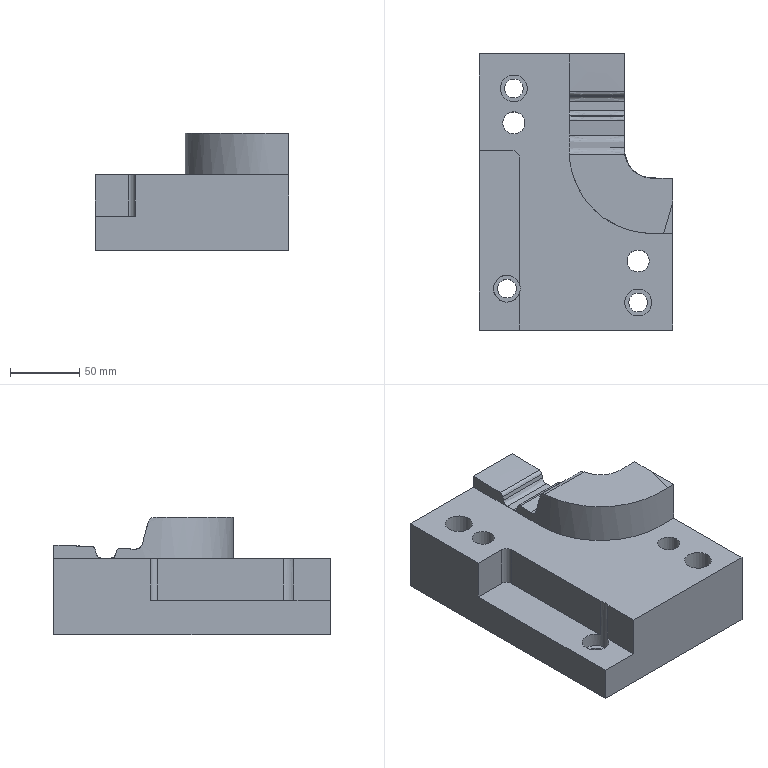Part | NX | features solid 2 | 1 solid | 40 faces | box 140 x 200 x 85 mm | volume 1309632 mm3 | spline 18 | plane 13 | cylinder 9 | commonest cylinder face diameters 13.5 x3 19.5 x3 16 x2 10 x1